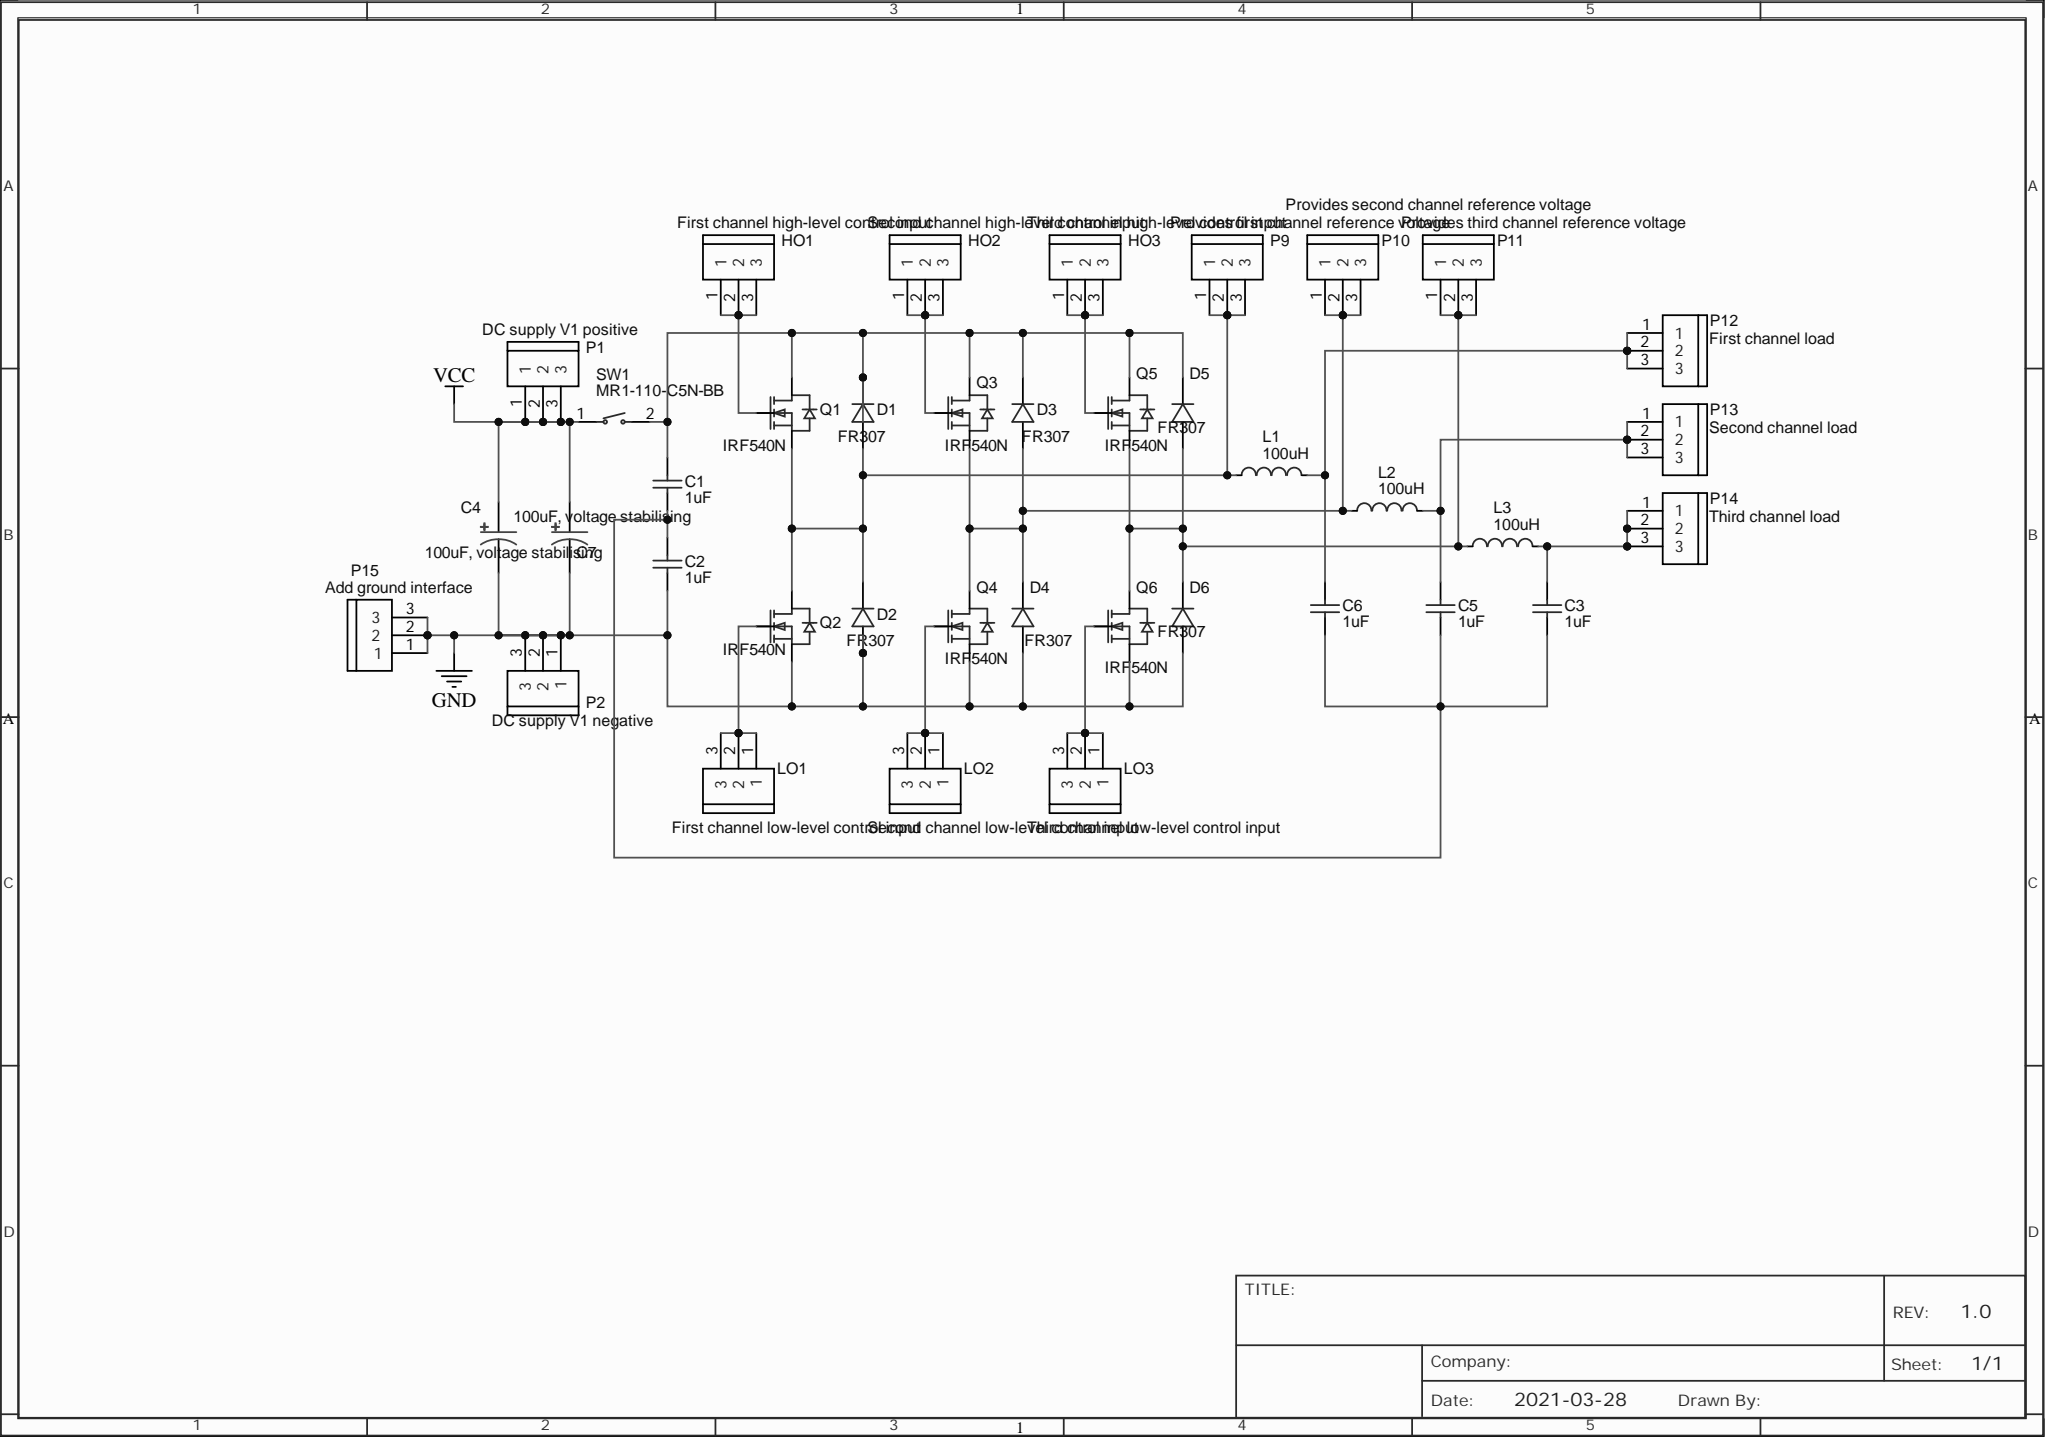Circuit board | Altium Designer | 38 parts | 16 nets
Bill of materials:
Comment,Description,Designator,Footprint,LibRef,Quantity
"1uF","","C1, C2, C3, C5, C6","CAP-TH_L18.0-W9.5-P15.00-D1.2","ECWF2W105KA","5"
"100uF, voltage stabilising","","C4, C7","CAP-TH_BD8.0-P3.50-D1.0-FD","SPV1HM101F11O00RAXXX","2"
"FR307","","D1, D2, D3, D4, D5, D6","DO-201AD_BD5.3-L8.4-P12.50-D1.4-RD","FR307","6"
"First channel high-level control input","","HO1","CONN-TH_3P-P5.00_WJ500V-5.08-3P","WJ500V-5.08-3P-14-00A","1"
"Second channel high-level control input","","HO2","CONN-TH_3P-P5.00_WJ500V-5.08-3P","WJ500V-5.08-3P-14-00A","1"
"Third channel high-level control input","","HO3","CONN-TH_3P-P5.00_WJ500V-5.08-3P","WJ500V-5.08-3P-14-00A","1"
"100uH","","L1, L2, L3","IND-SMD_L13.5-W12.6_125CDMCC-DS","TMPC1206HP-101MG-D","3"
"First channel low-level control input","","LO1","CONN-TH_3P-P5.00_WJ500V-5.08-3P","WJ500V-5.08-3P-14-00A","1"
"Second channel low-level control input","","LO2","CONN-TH_3P-P5.00_WJ500V-5.08-3P","WJ500V-5.08-3P-14-00A","1"
"Third channel low-level control input","","LO3","CONN-TH_3P-P5.00_WJ500V-5.08-3P","WJ500V-5.08-3P-14-00A","1"
"DC supply V1 positive","","P1","CONN-TH_3P-P5.00_WJ500V-5.08-3P","WJ500V-5.08-3P-14-00A","1"
"DC supply V1 negative","","P2","CONN-TH_3P-P5.00_WJ500V-5.08-3P","WJ500V-5.08-3P-14-00A","1"
"Provides first channel reference voltage","","P9","CONN-TH_3P-P5.00_WJ500V-5.08-3P","WJ500V-5.08-3P-14-00A","1"
"Provides second channel reference voltage","","P10","CONN-TH_3P-P5.00_WJ500V-5.08-3P","WJ500V-5.08-3P-14-00A","1"
"Provides third channel reference voltage","","P11","CONN-TH_3P-P5.00_WJ500V-5.08-3P","WJ500V-5.08-3P-14-00A","1"
"First channel load","","P12","CONN-TH_3P-P5.00_WJ500V-5.08-3P","WJ500V-5.08-3P-14-00A","1"
"Second channel load","","P13","CONN-TH_3P-P5.00_WJ500V-5.08-3P","WJ500V-5.08-3P-14-00A","1"
"Third channel load","","P14","CONN-TH_3P-P5.00_WJ500V-5.08-3P","WJ500V-5.08-3P-14-00A","1"
"Add ground interface","","P15","CONN-TH_3P-P5.00_WJ500V-5.08-3P","WJ500V-5.08-3P-14-00A","1"
"IRF540N","","Q1, Q2, Q3, Q4, Q5, Q6","TO-220AB-3_L10.4-W4.6-P2.54-L","IRF540N","6"
"MR1-110-C5N-BB","","SW1","SW-TH_MR1-110-C5N-BB","MR1-110-C5N-BB","1"
Netlist (Protel format):
[
C1
CAP-TH_L18.0-W9.5-P15.00-D1.2
1uF



]
[
C2
CAP-TH_L18.0-W9.5-P15.00-D1.2
1uF



]
[
C3
CAP-TH_L18.0-W9.5-P15.00-D1.2
1uF



]
[
C4
CAP-TH_BD8.0-P3.50-D1.0-FD
100uF, voltage stabilising



]
[
C5
CAP-TH_L18.0-W9.5-P15.00-D1.2
1uF



]
[
C6
CAP-TH_L18.0-W9.5-P15.00-D1.2
1uF



]
[
C7
CAP-TH_BD8.0-P3.50-D1.0-FD
100uF, voltage stabilising



]
[
D1
DO-201AD_BD5.3-L8.4-P12.50-D1.4-RD
FR307



]
[
D2
DO-201AD_BD5.3-L8.4-P12.50-D1.4-RD
FR307



]
[
D3
DO-201AD_BD5.3-L8.4-P12.50-D1.4-RD
FR307



]
[
D4
DO-201AD_BD5.3-L8.4-P12.50-D1.4-RD
FR307



]
[
D5
DO-201AD_BD5.3-L8.4-P12.50-D1.4-RD
FR307



]
[
D6
DO-201AD_BD5.3-L8.4-P12.50-D1.4-RD
FR307



]
[
HO1
CONN-TH_3P-P5.00_WJ500V-5.08-3P
First channel high-level control input



]
[
HO2
CONN-TH_3P-P5.00_WJ500V-5.08-3P
Second channel high-level control input



]
[
HO3
CONN-TH_3P-P5.00_WJ500V-5.08-3P
Third channel high-level control input



]
[
L1
IND-SMD_L13.5-W12.6_125CDMCC-DS
100uH



]
[
L2
IND-SMD_L13.5-W12.6_125CDMCC-DS
100uH



]
[
L3
IND-SMD_L13.5-W12.6_125CDMCC-DS
100uH



]
[
LO1
CONN-TH_3P-P5.00_WJ500V-5.08-3P
First channel low-level control input



]
[
LO2
CONN-TH_3P-P5.00_WJ500V-5.08-3P
Second channel low-level control input



]
[
LO3
CONN-TH_3P-P5.00_WJ500V-5.08-3P
Third channel low-level control input



]
[
P1
CONN-TH_3P-P5.00_WJ500V-5.08-3P
DC supply V1 positive



]
[
P2
CONN-TH_3P-P5.00_WJ500V-5.08-3P
DC supply V1 negative



]
[
P9
CONN-TH_3P-P5.00_WJ500V-5.08-3P
Provides first channel reference voltage



]
[
P10
CONN-TH_3P-P5.00_WJ500V-5.08-3P
Provides second channel reference voltage



]
[
P11
CONN-TH_3P-P5.00_WJ500V-5.08-3P
Provides third channel reference voltage



]
[
P12
CONN-TH_3P-P5.00_WJ500V-5.08-3P
First channel load



]
[
P13
CONN-TH_3P-P5.00_WJ500V-5.08-3P
Second channel load



]
[
P14
CONN-TH_3P-P5.00_WJ500V-5.08-3P
Third channel load



]
[
P15
CONN-TH_3P-P5.00_WJ500V-5.08-3P
Add ground interface



]
[
Q1
TO-220AB-3_L10.4-W4.6-P2.54-L
IRF540N



]
[
Q2
TO-220AB-3_L10.4-W4.6-P2.54-L
IRF540N



]
[
Q3
TO-220AB-3_L10.4-W4.6-P2.54-L
IRF540N



]
[
Q4
TO-220AB-3_L10.4-W4.6-P2.54-L
IRF540N



]
[
Q5
TO-220AB-3_L10.4-W4.6-P2.54-L
IRF540N



]
[
Q6
TO-220AB-3_L10.4-W4.6-P2.54-L
IRF540N



]
[
SW1
SW-TH_MR1-110-C5N-BB
MR1-110-C5N-BB



]
(
VCC
C4-1
C7-1
P1-1
P1-2
P1-3
SW1-1
)
(
NetLO3_1
LO3-1
LO3-2
LO3-3
Q6-1
)
(
NetLO2_1
LO2-1
LO2-2
LO2-3
Q4-1
)
(
NetLO1_1
LO1-1
LO1-2
LO1-3
Q2-1
)
(
NetHO3_1
HO3-1
HO3-2
HO3-3
Q5-1
)
(
NetHO2_1
HO2-1
HO2-2
HO2-3
Q3-1
)
(
NetHO1_1
HO1-1
HO1-2
HO1-3
Q1-1
)
(
NetD5_2
D5-2
D6-1
L3-1
P11-1
P11-2
P11-3
Q5-3
Q6-2
)
(
NetD3_2
D3-2
D4-1
L2-1
P10-1
P10-2
P10-3
Q3-3
Q4-2
)
(
NetD1_2
D1-2
D2-1
L1-1
P9-1
P9-2
P9-3
Q1-3
Q2-2
)
(
NetC6_2
C6-2
L1-2
P12-1
P12-2
P12-3
)
(
NetC5_2
C5-2
L2-2
P13-1
P13-2
P13-3
)
(
NetC3_2
C3-2
L3-2
P14-1
P14-2
P14-3
)
(
NetC1_2
C1-2
D1-1
D3-1
D5-1
Q1-2
Q3-2
Q5-2
SW1-2
)
(
NetC1_1
C1-1
C2-2
C3-1
C5-1
C6-1
)
(
GND
C2-1
C4-2
C7-2
D2-2
D4-2
D6-2
P2-1
P2-2
P2-3
P15-1
P15-2
P15-3
Q2-3
Q4-3
Q6-3
)